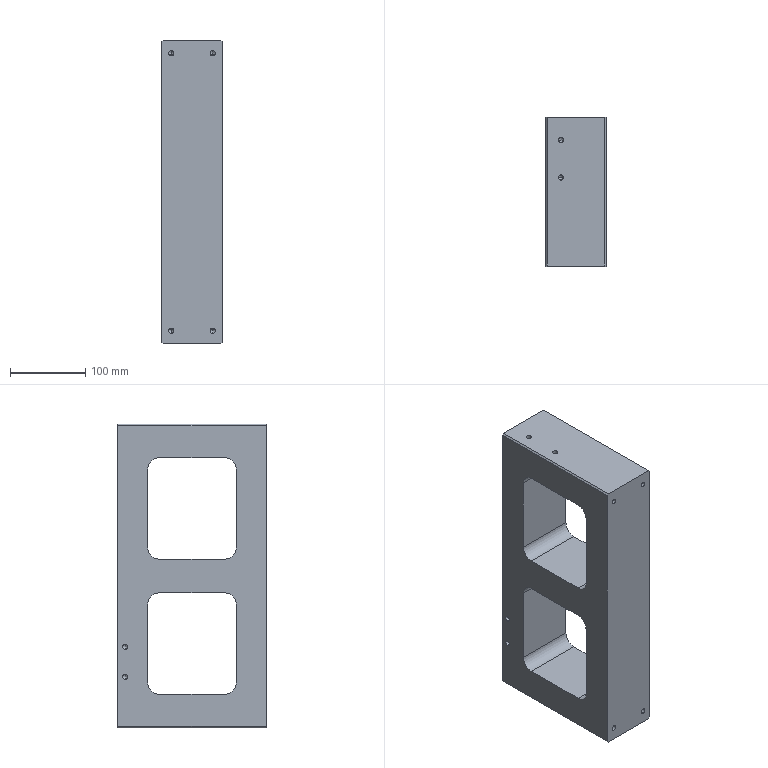Part | SolidWorks | features BaseBody 1 | 1 solid | 74 faces | box 80 x 198 x 405 mm | volume 3883982 mm3 | cylinder 32 | cone 24 | plane 18 | commonest cylinder face diameters 6.8 x24 30 x8